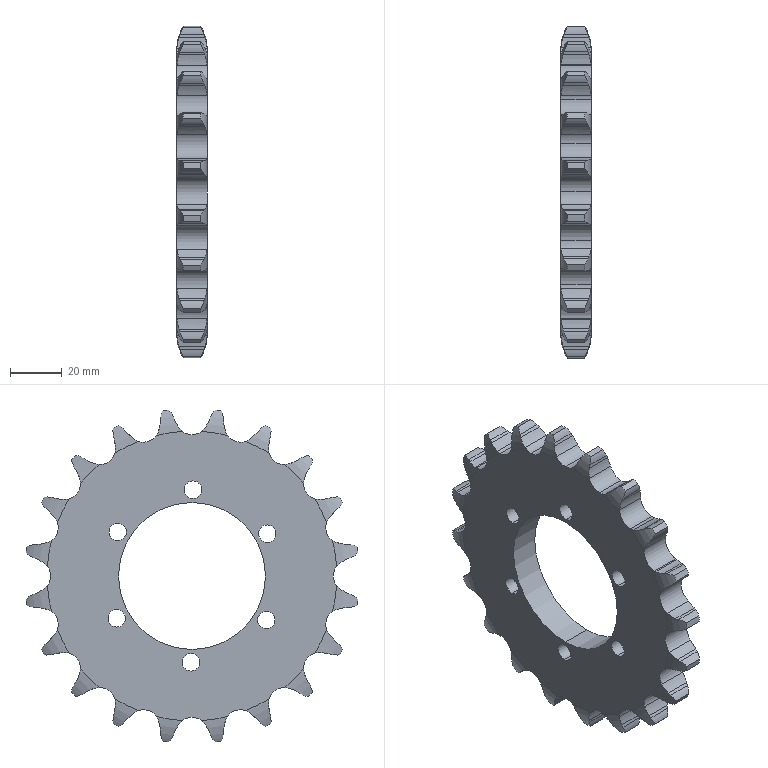Part | SolidWorks | features BaseBody 1 | 1 solid | 225 faces | box 11.69 x 128.76 x 128.76 mm | volume 93096 mm3 | cylinder 143 | plane 42 | spline 40 | commonest cylinder face diameters 17.336 x42 31.126 x42 12.07 x25 130 x20 6.8 x12 57 x2